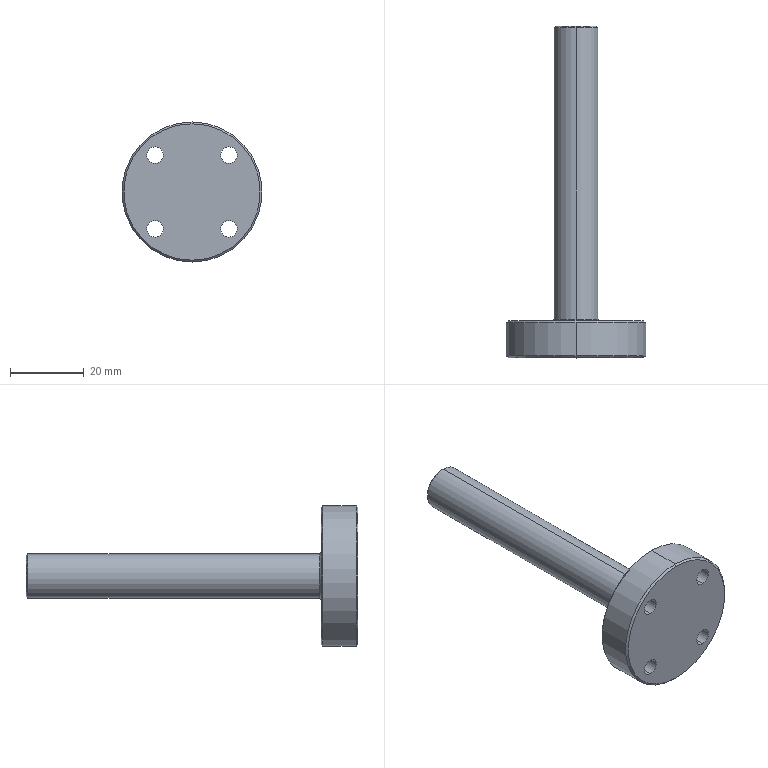Part | STEP file | ND25021-01-JDKM-10-GJ | 1 solid | 23 faces | box 38 x 90 x 38 mm | volume 19721 mm3 | cylinder 12 | cone 6 | plane 3 | torus 2 | commonest cylinder face diameters 4.5 x8 12 x2 38 x2